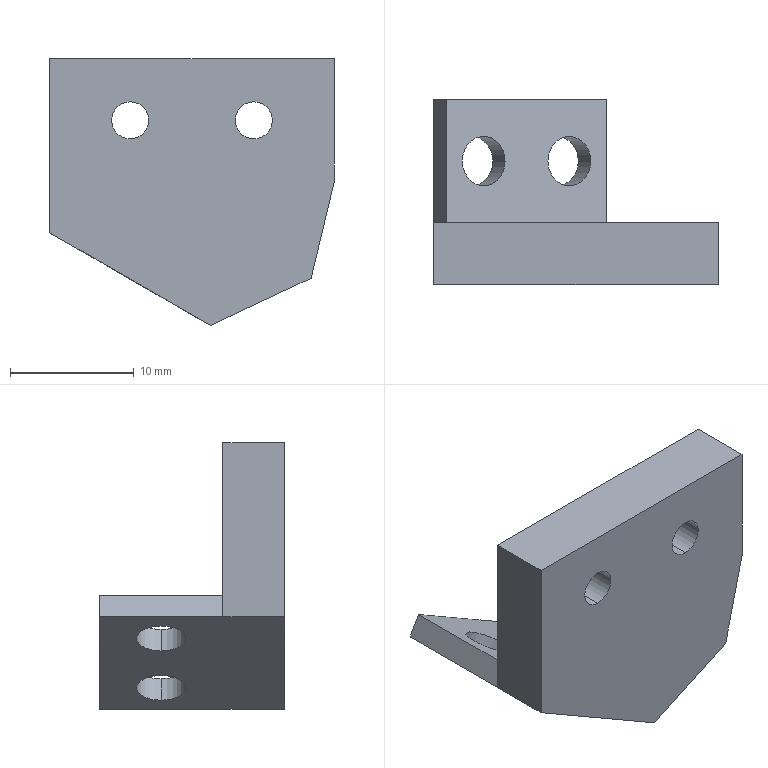Part | SolidWorks | features ICE 3, Extrusion 1 | 1 solid | 20 faces | box 23 x 15 x 21.606 mm | volume 2270 mm3 | plane 12 | cylinder 8 | commonest cylinder face diameters 3 x4 4 x4
STEP:
#1=CARTESIAN_POINT('',(-16.5,0.,-6.5));
#2=VERTEX_POINT('',#1);
#3=CARTESIAN_POINT('',(-16.5,0.,-3.5));
#4=VERTEX_POINT('',#3);
#5=CARTESIAN_POINT('',(-16.5,0.,-5.));
#6=DIRECTION('',(0.,1.,0.));
#7=DIRECTION('',(0.,0.,1.));
#8=AXIS2_PLACEMENT_3D('',#5,#6,#7);
#9=CIRCLE('',#8,1.5);
#10=EDGE_CURVE('',#2,#4,#9,.T.);
#11=ORIENTED_EDGE('',*,*,#10,.F.);
#12=CARTESIAN_POINT('',(-16.5,5.,-6.5));
#13=VERTEX_POINT('',#12);
#14=CARTESIAN_POINT('',(-16.5,0.,-6.5));
#15=DIRECTION('',(0.,1.,0.));
#16=VECTOR('',#15,1000.);
#17=LINE('',#14,#16);
#18=EDGE_CURVE('',#2,#13,#17,.T.);
#19=ORIENTED_EDGE('',*,*,#18,.T.);
#20=CARTESIAN_POINT('',(-16.5,5.,-3.5));
#21=VERTEX_POINT('',#20);
#22=CARTESIAN_POINT('',(-16.5,5.,-5.));
#23=DIRECTION('',(0.,-1.,0.));
#24=DIRECTION('',(0.,0.,-1.));
#25=AXIS2_PLACEMENT_3D('',#22,#23,#24);
#26=CIRCLE('',#25,1.5);
#27=EDGE_CURVE('',#21,#13,#26,.T.);
#28=ORIENTED_EDGE('',*,*,#27,.F.);
#29=CARTESIAN_POINT('',(-16.5,0.,-3.5));
#30=DIRECTION('',(0.,1.,0.));
#31=VECTOR('',#30,1000.);
#32=LINE('',#29,#31);
#33=EDGE_CURVE('',#4,#21,#32,.T.);
#34=ORIENTED_EDGE('',*,*,#33,.F.);
#35=EDGE_LOOP('',(#11,#19,#28,#34));
#36=FACE_OUTER_BOUND('',#35,.T.);
#37=CARTESIAN_POINT('',(-16.5,0.,-5.));
#38=DIRECTION('',(0.,1.,0.));
#39=DIRECTION('',(0.,0.,1.));
#40=AXIS2_PLACEMENT_3D('',#37,#38,#39);
#41=CYLINDRICAL_SURFACE('',#40,1.5);
#42=ADVANCED_FACE('',(#36),#41,.F.);
#43=CARTESIAN_POINT('',(-6.5,0.,-6.5));
#44=VERTEX_POINT('',#43);
#45=CARTESIAN_POINT('',(-6.5,0.,-3.5));
#46=VERTEX_POINT('',#45);
#47=CARTESIAN_POINT('',(-6.5,0.,-5.));
#48=DIRECTION('',(0.,1.,0.));
#49=DIRECTION('',(0.,0.,1.));
#50=AXIS2_PLACEMENT_3D('',#47,#48,#49);
#51=CIRCLE('',#50,1.5);
#52=EDGE_CURVE('',#44,#46,#51,.T.);
#53=ORIENTED_EDGE('',*,*,#52,.F.);
#54=CARTESIAN_POINT('',(-6.5,5.,-6.5));
#55=VERTEX_POINT('',#54);
#56=CARTESIAN_POINT('',(-6.5,0.,-6.5));
#57=DIRECTION('',(0.,1.,0.));
#58=VECTOR('',#57,1000.);
#59=LINE('',#56,#58);
#60=EDGE_CURVE('',#44,#55,#59,.T.);
#61=ORIENTED_EDGE('',*,*,#60,.T.);
#62=CARTESIAN_POINT('',(-6.5,5.,-3.5));
#63=VERTEX_POINT('',#62);
#64=CARTESIAN_POINT('',(-6.5,5.,-5.));
#65=DIRECTION('',(0.,-1.,0.));
#66=DIRECTION('',(0.,0.,-1.));
#67=AXIS2_PLACEMENT_3D('',#64,#65,#66);
#68=CIRCLE('',#67,1.5);
#69=EDGE_CURVE('',#63,#55,#68,.T.);
#70=ORIENTED_EDGE('',*,*,#69,.F.);
#71=CARTESIAN_POINT('',(-6.5,0.,-3.5));
#72=DIRECTION('',(0.,1.,0.));
#73=VECTOR('',#72,1000.);
#74=LINE('',#71,#73);
#75=EDGE_CURVE('',#46,#63,#74,.T.);
#76=ORIENTED_EDGE('',*,*,#75,.F.);
#77=EDGE_LOOP('',(#53,#61,#70,#76));
#78=FACE_OUTER_BOUND('',#77,.T.);
#79=CARTESIAN_POINT('',(-6.5,0.,-5.));
#80=DIRECTION('',(0.,1.,0.));
#81=DIRECTION('',(0.,0.,1.));
#82=AXIS2_PLACEMENT_3D('',#79,#80,#81);
#83=CYLINDRICAL_SURFACE('',#82,1.5);
#84=ADVANCED_FACE('',(#78),#83,.F.);
#85=CARTESIAN_POINT('',(-14.773,10.,-18.856));
#86=VERTEX_POINT('',#85);
#87=CARTESIAN_POINT('',(-11.309,10.,-20.856));
#88=VERTEX_POINT('',#87);
#89=CARTESIAN_POINT('',(-13.041,10.,-19.856));
#90=DIRECTION('',(0.5,0.,0.866));
#91=DIRECTION('',(0.866,0.,-0.5));
#92=AXIS2_PLACEMENT_3D('',#89,#90,#91);
#93=CIRCLE('',#92,2.);
#94=EDGE_CURVE('',#86,#88,#93,.T.);
#95=ORIENTED_EDGE('',*,*,#94,.F.);
#96=CARTESIAN_POINT('',(-13.773,10.,-17.124));
#97=VERTEX_POINT('',#96);
#98=CARTESIAN_POINT('',(-18.02,10.,-24.481));
#99=DIRECTION('',(0.5,0.,0.866));
#100=VECTOR('',#99,1000.);
#101=LINE('',#98,#100);
#102=EDGE_CURVE('',#86,#97,#101,.T.);
#103=ORIENTED_EDGE('',*,*,#102,.T.);
#104=CARTESIAN_POINT('',(-10.309,10.,-19.124));
#105=VERTEX_POINT('',#104);
#106=CARTESIAN_POINT('',(-12.041,10.,-18.124));
#107=DIRECTION('',(-0.5,0.,-0.866));
#108=DIRECTION('',(-0.866,0.,0.5));
#109=AXIS2_PLACEMENT_3D('',#106,#107,#108);
#110=CIRCLE('',#109,2.);
#111=EDGE_CURVE('',#105,#97,#110,.T.);
#112=ORIENTED_EDGE('',*,*,#111,.F.);
#113=CARTESIAN_POINT('',(-14.556,10.,-26.481));
#114=DIRECTION('',(0.5,0.,0.866));
#115=VECTOR('',#114,1000.);
#116=LINE('',#113,#115);
#117=EDGE_CURVE('',#88,#105,#116,.T.);
#118=ORIENTED_EDGE('',*,*,#117,.F.);
#119=EDGE_LOOP('',(#95,#103,#112,#118));
#120=FACE_OUTER_BOUND('',#119,.T.);
#121=CARTESIAN_POINT('',(-16.288,10.,-25.481));
#122=DIRECTION('',(0.5,0.,0.866));
#123=DIRECTION('',(0.866,0.,-0.5));
#124=AXIS2_PLACEMENT_3D('',#121,#122,#123);
#125=CYLINDRICAL_SURFACE('',#124,2.);
#126=ADVANCED_FACE('',(#120),#125,.F.);
#127=CARTESIAN_POINT('',(-21.701,10.,-14.856));
#128=VERTEX_POINT('',#127);
#129=CARTESIAN_POINT('',(-18.237,10.,-16.856));
#130=VERTEX_POINT('',#129);
#131=CARTESIAN_POINT('',(-19.969,10.,-15.856));
#132=DIRECTION('',(0.5,0.,0.866));
#133=DIRECTION('',(0.866,0.,-0.5));
#134=AXIS2_PLACEMENT_3D('',#131,#132,#133);
#135=CIRCLE('',#134,2.);
#136=EDGE_CURVE('',#128,#130,#135,.T.);
#137=ORIENTED_EDGE('',*,*,#136,.F.);
#138=CARTESIAN_POINT('',(-20.701,10.,-13.124));
#139=VERTEX_POINT('',#138);
#140=CARTESIAN_POINT('',(-24.949,10.,-20.481));
#141=DIRECTION('',(0.5,0.,0.866));
#142=VECTOR('',#141,1000.);
#143=LINE('',#140,#142);
#144=EDGE_CURVE('',#128,#139,#143,.T.);
#145=ORIENTED_EDGE('',*,*,#144,.T.);
#146=CARTESIAN_POINT('',(-17.237,10.,-15.124));
#147=VERTEX_POINT('',#146);
#148=CARTESIAN_POINT('',(-18.969,10.,-14.124));
#149=DIRECTION('',(-0.5,0.,-0.866));
#150=DIRECTION('',(-0.866,0.,0.5));
#151=AXIS2_PLACEMENT_3D('',#148,#149,#150);
#152=CIRCLE('',#151,2.);
#153=EDGE_CURVE('',#147,#139,#152,.T.);
#154=ORIENTED_EDGE('',*,*,#153,.F.);
#155=CARTESIAN_POINT('',(-21.484,10.,-22.481));
#156=DIRECTION('',(0.5,0.,0.866));
#157=VECTOR('',#156,1000.);
#158=LINE('',#155,#157);
#159=EDGE_CURVE('',#130,#147,#158,.T.);
#160=ORIENTED_EDGE('',*,*,#159,.F.);
#161=EDGE_LOOP('',(#137,#145,#154,#160));
#162=FACE_OUTER_BOUND('',#161,.T.);
#163=CARTESIAN_POINT('',(-23.217,10.,-21.481));
#164=DIRECTION('',(0.5,0.,0.866));
#165=DIRECTION('',(0.866,0.,-0.5));
#166=AXIS2_PLACEMENT_3D('',#163,#164,#165);
#167=CYLINDRICAL_SURFACE('',#166,2.);
#168=ADVANCED_FACE('',(#162),#167,.F.);
#169=ORIENTED_EDGE('',*,*,#27,.T.);
#170=CARTESIAN_POINT('',(-16.5,5.,-5.));
#171=DIRECTION('',(0.,-1.,0.));
#172=DIRECTION('',(0.,0.,-1.));
#173=AXIS2_PLACEMENT_3D('',#170,#171,#172);
#174=CIRCLE('',#173,1.5);
#175=EDGE_CURVE('',#13,#21,#174,.T.);
#176=ORIENTED_EDGE('',*,*,#175,.T.);
#177=EDGE_LOOP('',(#169,#176));
#178=FACE_BOUND('',#177,.T.);
#179=ORIENTED_EDGE('',*,*,#69,.T.);
#180=CARTESIAN_POINT('',(-6.5,5.,-5.));
#181=DIRECTION('',(0.,-1.,0.));
#182=DIRECTION('',(0.,0.,-1.));
#183=AXIS2_PLACEMENT_3D('',#180,#181,#182);
#184=CIRCLE('',#183,1.5);
#185=EDGE_CURVE('',#55,#63,#184,.T.);
#186=ORIENTED_EDGE('',*,*,#185,.T.);
#187=EDGE_LOOP('',(#179,#186));
#188=FACE_BOUND('',#187,.T.);
#189=CARTESIAN_POINT('',(-9.01,5.,-19.874));
#190=VERTEX_POINT('',#189);
#191=CARTESIAN_POINT('',(-10.01,5.,-21.606));
#192=VERTEX_POINT('',#191);
#193=CARTESIAN_POINT('',(-10.01,5.,-21.606));
#194=DIRECTION('',(-0.5,0.,-0.866));
#195=VECTOR('',#194,1000.);
#196=LINE('',#193,#195);
#197=EDGE_CURVE('',#190,#192,#196,.T.);
#198=ORIENTED_EDGE('',*,*,#197,.F.);
#199=CARTESIAN_POINT('',(-22.,5.,-12.374));
#200=VERTEX_POINT('',#199);
#201=CARTESIAN_POINT('',(-22.,5.,-12.374));
#202=DIRECTION('',(0.866,0.,-0.5));
#203=VECTOR('',#202,1000.);
#204=LINE('',#201,#203);
#205=EDGE_CURVE('',#200,#190,#204,.T.);
#206=ORIENTED_EDGE('',*,*,#205,.F.);
#207=CARTESIAN_POINT('',(-23.,5.,-14.106));
#208=VERTEX_POINT('',#207);
#209=CARTESIAN_POINT('',(-23.,5.,-14.106));
#210=DIRECTION('',(0.5,0.,0.866));
#211=VECTOR('',#210,1000.);
#212=LINE('',#209,#211);
#213=EDGE_CURVE('',#208,#200,#212,.T.);
#214=ORIENTED_EDGE('',*,*,#213,.F.);
#215=CARTESIAN_POINT('',(-23.,5.,0.));
#216=VERTEX_POINT('',#215);
#217=CARTESIAN_POINT('',(-23.,5.,0.));
#218=DIRECTION('',(0.,0.,1.));
#219=VECTOR('',#218,1000.);
#220=LINE('',#217,#219);
#221=EDGE_CURVE('',#208,#216,#220,.T.);
#222=ORIENTED_EDGE('',*,*,#221,.T.);
#223=CARTESIAN_POINT('',(0.,5.,0.));
#224=VERTEX_POINT('',#223);
#225=CARTESIAN_POINT('',(0.,5.,0.));
#226=DIRECTION('',(1.,0.,0.));
#227=VECTOR('',#226,1000.);
#228=LINE('',#225,#227);
#229=EDGE_CURVE('',#216,#224,#228,.T.);
#230=ORIENTED_EDGE('',*,*,#229,.T.);
#231=CARTESIAN_POINT('',(0.,5.,-10.));
#232=VERTEX_POINT('',#231);
#233=CARTESIAN_POINT('',(0.,5.,-10.));
#234=DIRECTION('',(0.,0.,-1.));
#235=VECTOR('',#234,1000.);
#236=LINE('',#233,#235);
#237=EDGE_CURVE('',#224,#232,#236,.T.);
#238=ORIENTED_EDGE('',*,*,#237,.T.);
#239=CARTESIAN_POINT('',(-1.863,5.,-17.78));
#240=VERTEX_POINT('',#239);
#241=CARTESIAN_POINT('',(-1.863,5.,-17.78));
#242=DIRECTION('',(-0.2329,0.,-0.9725));
#243=VECTOR('',#242,1000.);
#244=LINE('',#241,#243);
#245=EDGE_CURVE('',#232,#240,#244,.T.);
#246=ORIENTED_EDGE('',*,*,#245,.T.);
#247=CARTESIAN_POINT('',(-10.01,5.,-21.606));
#248=DIRECTION('',(-0.9052,0.,-0.4251));
#249=VECTOR('',#248,1000.);
#250=LINE('',#247,#249);
#251=EDGE_CURVE('',#240,#192,#250,.T.);
#252=ORIENTED_EDGE('',*,*,#251,.T.);
#253=EDGE_LOOP('',(#198,#206,#214,#222,#230,#238,#246,#252));
#254=FACE_OUTER_BOUND('',#253,.T.);
#255=CARTESIAN_POINT('',(0.,5.,0.));
#256=DIRECTION('',(0.,-1.,0.));
#257=DIRECTION('',(0.,0.,-1.));
#258=AXIS2_PLACEMENT_3D('',#255,#256,#257);
#259=PLANE('',#258);
#260=ADVANCED_FACE('',(#178,#188,#254),#259,.F.);
#261=CARTESIAN_POINT('',(0.,0.,0.));
#262=VERTEX_POINT('',#261);
#263=CARTESIAN_POINT('',(0.,0.,-10.));
#264=VERTEX_POINT('',#263);
#265=CARTESIAN_POINT('',(0.,0.,-10.));
#266=DIRECTION('',(0.,0.,-1.));
#267=VECTOR('',#266,1000.);
#268=LINE('',#265,#267);
#269=EDGE_CURVE('',#262,#264,#268,.T.);
#270=ORIENTED_EDGE('',*,*,#269,.T.);
#271=CARTESIAN_POINT('',(0.,5.,-10.));
#272=DIRECTION('',(0.,-1.,0.));
#273=VECTOR('',#272,1000.);
#274=LINE('',#271,#273);
#275=EDGE_CURVE('',#232,#264,#274,.T.);
#276=ORIENTED_EDGE('',*,*,#275,.F.);
#277=ORIENTED_EDGE('',*,*,#237,.F.);
#278=CARTESIAN_POINT('',(0.,5.,0.));
#279=DIRECTION('',(0.,-1.,0.));
#280=VECTOR('',#279,1000.);
#281=LINE('',#278,#280);
#282=EDGE_CURVE('',#224,#262,#281,.T.);
#283=ORIENTED_EDGE('',*,*,#282,.T.);
#284=EDGE_LOOP('',(#270,#276,#277,#283));
#285=FACE_OUTER_BOUND('',#284,.T.);
#286=CARTESIAN_POINT('',(0.,5.,-10.));
#287=DIRECTION('',(-1.,0.,0.));
#288=DIRECTION('',(0.,0.,1.));
#289=AXIS2_PLACEMENT_3D('',#286,#287,#288);
#290=PLANE('',#289);
#291=ADVANCED_FACE('',(#285),#290,.F.);
#292=CARTESIAN_POINT('',(-1.863,0.,-17.78));
#293=VERTEX_POINT('',#292);
#294=CARTESIAN_POINT('',(-1.863,0.,-17.78));
#295=DIRECTION('',(-0.2329,0.,-0.9725));
#296=VECTOR('',#295,1000.);
#297=LINE('',#294,#296);
#298=EDGE_CURVE('',#264,#293,#297,.T.);
#299=ORIENTED_EDGE('',*,*,#298,.T.);
#300=CARTESIAN_POINT('',(-1.863,5.,-17.78));
#301=DIRECTION('',(0.,-1.,0.));
#302=VECTOR('',#301,1000.);
#303=LINE('',#300,#302);
#304=EDGE_CURVE('',#240,#293,#303,.T.);
#305=ORIENTED_EDGE('',*,*,#304,.F.);
#306=ORIENTED_EDGE('',*,*,#245,.F.);
#307=ORIENTED_EDGE('',*,*,#275,.T.);
#308=EDGE_LOOP('',(#299,#305,#306,#307));
#309=FACE_OUTER_BOUND('',#308,.T.);
#310=CARTESIAN_POINT('',(-1.863,5.,-17.78));
#311=DIRECTION('',(-0.9725,0.,0.2329));
#312=DIRECTION('',(0.2329,0.,0.9725));
#313=AXIS2_PLACEMENT_3D('',#310,#311,#312);
#314=PLANE('',#313);
#315=ADVANCED_FACE('',(#309),#314,.F.);
#316=CARTESIAN_POINT('',(-10.01,0.,-21.606));
#317=VERTEX_POINT('',#316);
#318=CARTESIAN_POINT('',(-10.01,0.,-21.606));
#319=DIRECTION('',(-0.9052,0.,-0.4251));
#320=VECTOR('',#319,1000.);
#321=LINE('',#318,#320);
#322=EDGE_CURVE('',#293,#317,#321,.T.);
#323=ORIENTED_EDGE('',*,*,#322,.T.);
#324=CARTESIAN_POINT('',(-10.01,5.,-21.606));
#325=DIRECTION('',(0.,-1.,0.));
#326=VECTOR('',#325,1000.);
#327=LINE('',#324,#326);
#328=EDGE_CURVE('',#192,#317,#327,.T.);
#329=ORIENTED_EDGE('',*,*,#328,.F.);
#330=ORIENTED_EDGE('',*,*,#251,.F.);
#331=ORIENTED_EDGE('',*,*,#304,.T.);
#332=EDGE_LOOP('',(#323,#329,#330,#331));
#333=FACE_OUTER_BOUND('',#332,.T.);
#334=CARTESIAN_POINT('',(-10.01,5.,-21.606));
#335=DIRECTION('',(-0.4251,0.,0.9052));
#336=DIRECTION('',(0.9052,0.,0.4251));
#337=AXIS2_PLACEMENT_3D('',#334,#335,#336);
#338=PLANE('',#337);
#339=ADVANCED_FACE('',(#333),#338,.F.);
#340=CARTESIAN_POINT('',(-13.041,10.,-19.856));
#341=DIRECTION('',(0.5,0.,0.866));
#342=DIRECTION('',(0.866,0.,-0.5));
#343=AXIS2_PLACEMENT_3D('',#340,#341,#342);
#344=CIRCLE('',#343,2.);
#345=EDGE_CURVE('',#88,#86,#344,.T.);
#346=ORIENTED_EDGE('',*,*,#345,.T.);
#347=ORIENTED_EDGE('',*,*,#94,.T.);
#348=EDGE_LOOP('',(#346,#347));
#349=FACE_BOUND('',#348,.T.);
#350=CARTESIAN_POINT('',(-19.969,10.,-15.856));
#351=DIRECTION('',(0.5,0.,0.866));
#352=DIRECTION('',(0.866,0.,-0.5));
#353=AXIS2_PLACEMENT_3D('',#350,#351,#352);
#354=CIRCLE('',#353,2.);
#355=EDGE_CURVE('',#130,#128,#354,.T.);
#356=ORIENTED_EDGE('',*,*,#355,.T.);
#357=ORIENTED_EDGE('',*,*,#136,.T.);
#358=EDGE_LOOP('',(#356,#357));
#359=FACE_BOUND('',#358,.T.);
#360=CARTESIAN_POINT('',(-23.,0.,-14.106));
#361=VERTEX_POINT('',#360);
#362=CARTESIAN_POINT('',(-23.,0.,-14.106));
#363=DIRECTION('',(-0.866,0.,0.5));
#364=VECTOR('',#363,1000.);
#365=LINE('',#362,#364);
#366=EDGE_CURVE('',#317,#361,#365,.T.);
#367=ORIENTED_EDGE('',*,*,#366,.T.);
#368=CARTESIAN_POINT('',(-23.,5.,-14.106));
#369=DIRECTION('',(0.,-1.,0.));
#370=VECTOR('',#369,1000.);
#371=LINE('',#368,#370);
#372=EDGE_CURVE('',#208,#361,#371,.T.);
#373=ORIENTED_EDGE('',*,*,#372,.F.);
#374=CARTESIAN_POINT('',(-23.,15.,-14.106));
#375=VERTEX_POINT('',#374);
#376=CARTESIAN_POINT('',(-23.,15.,-14.106));
#377=DIRECTION('',(0.,-1.,0.));
#378=VECTOR('',#377,1000.);
#379=LINE('',#376,#378);
#380=EDGE_CURVE('',#375,#208,#379,.T.);
#381=ORIENTED_EDGE('',*,*,#380,.F.);
#382=CARTESIAN_POINT('',(-10.01,15.,-21.606));
#383=VERTEX_POINT('',#382);
#384=CARTESIAN_POINT('',(-10.01,15.,-21.606));
#385=DIRECTION('',(-0.866,0.,0.5));
#386=VECTOR('',#385,1000.);
#387=LINE('',#384,#386);
#388=EDGE_CURVE('',#383,#375,#387,.T.);
#389=ORIENTED_EDGE('',*,*,#388,.F.);
#390=CARTESIAN_POINT('',(-10.01,15.,-21.606));
#391=DIRECTION('',(0.,-1.,0.));
#392=VECTOR('',#391,1000.);
#393=LINE('',#390,#392);
#394=EDGE_CURVE('',#383,#192,#393,.T.);
#395=ORIENTED_EDGE('',*,*,#394,.T.);
#396=ORIENTED_EDGE('',*,*,#328,.T.);
#397=EDGE_LOOP('',(#367,#373,#381,#389,#395,#396));
#398=FACE_OUTER_BOUND('',#397,.T.);
#399=CARTESIAN_POINT('',(-23.,5.,-14.106));
#400=DIRECTION('',(0.5,0.,0.866));
#401=DIRECTION('',(0.866,0.,-0.5));
#402=AXIS2_PLACEMENT_3D('',#399,#400,#401);
#403=PLANE('',#402);
#404=ADVANCED_FACE('',(#349,#359,#398),#403,.F.);
#405=CARTESIAN_POINT('',(-23.,0.,0.));
#406=VERTEX_POINT('',#405);
#407=CARTESIAN_POINT('',(-23.,0.,0.));
#408=DIRECTION('',(0.,0.,1.));
#409=VECTOR('',#408,1000.);
#410=LINE('',#407,#409);
#411=EDGE_CURVE('',#361,#406,#410,.T.);
#412=ORIENTED_EDGE('',*,*,#411,.T.);
#413=CARTESIAN_POINT('',(-23.,5.,0.));
#414=DIRECTION('',(0.,-1.,0.));
#415=VECTOR('',#414,1000.);
#416=LINE('',#413,#415);
#417=EDGE_CURVE('',#216,#406,#416,.T.);
#418=ORIENTED_EDGE('',*,*,#417,.F.);
#419=ORIENTED_EDGE('',*,*,#221,.F.);
#420=ORIENTED_EDGE('',*,*,#372,.T.);
#421=EDGE_LOOP('',(#412,#418,#419,#420));
#422=FACE_OUTER_BOUND('',#421,.T.);
#423=CARTESIAN_POINT('',(-23.,5.,0.));
#424=DIRECTION('',(1.,0.,0.));
#425=DIRECTION('',(0.,0.,-1.));
#426=AXIS2_PLACEMENT_3D('',#423,#424,#425);
#427=PLANE('',#426);
#428=ADVANCED_FACE('',(#422),#427,.F.);
#429=CARTESIAN_POINT('',(0.,0.,0.));
#430=DIRECTION('',(1.,0.,0.));
#431=VECTOR('',#430,1000.);
#432=LINE('',#429,#431);
#433=EDGE_CURVE('',#406,#262,#432,.T.);
#434=ORIENTED_EDGE('',*,*,#433,.T.);
#435=ORIENTED_EDGE('',*,*,#282,.F.);
#436=ORIENTED_EDGE('',*,*,#229,.F.);
#437=ORIENTED_EDGE('',*,*,#417,.T.);
#438=EDGE_LOOP('',(#434,#435,#436,#437));
#439=FACE_OUTER_BOUND('',#438,.T.);
#440=CARTESIAN_POINT('',(0.,5.,0.));
#441=DIRECTION('',(0.,0.,-1.));
#442=DIRECTION('',(-1.,0.,0.));
#443=AXIS2_PLACEMENT_3D('',#440,#441,#442);
#444=PLANE('',#443);
#445=ADVANCED_FACE('',(#439),#444,.F.);
#446=CARTESIAN_POINT('',(-16.5,0.,-5.));
#447=DIRECTION('',(0.,1.,0.));
#448=DIRECTION('',(0.,0.,1.));
#449=AXIS2_PLACEMENT_3D('',#446,#447,#448);
#450=CIRCLE('',#449,1.5);
#451=EDGE_CURVE('',#4,#2,#450,.T.);
#452=ORIENTED_EDGE('',*,*,#451,.T.);
#453=ORIENTED_EDGE('',*,*,#10,.T.);
#454=EDGE_LOOP('',(#452,#453));
#455=FACE_BOUND('',#454,.T.);
#456=CARTESIAN_POINT('',(-6.5,0.,-5.));
#457=DIRECTION('',(0.,1.,0.));
#458=DIRECTION('',(0.,0.,1.));
#459=AXIS2_PLACEMENT_3D('',#456,#457,#458);
#460=CIRCLE('',#459,1.5);
#461=EDGE_CURVE('',#46,#44,#460,.T.);
#462=ORIENTED_EDGE('',*,*,#461,.T.);
#463=ORIENTED_EDGE('',*,*,#52,.T.);
#464=EDGE_LOOP('',(#462,#463));
#465=FACE_BOUND('',#464,.T.);
#466=ORIENTED_EDGE('',*,*,#269,.F.);
#467=ORIENTED_EDGE('',*,*,#433,.F.);
#468=ORIENTED_EDGE('',*,*,#411,.F.);
#469=ORIENTED_EDGE('',*,*,#366,.F.);
#470=ORIENTED_EDGE('',*,*,#322,.F.);
#471=ORIENTED_EDGE('',*,*,#298,.F.);
#472=EDGE_LOOP('',(#466,#467,#468,#469,#470,#471));
#473=FACE_OUTER_BOUND('',#472,.T.);
#474=CARTESIAN_POINT('',(0.,0.,0.));
#475=DIRECTION('',(0.,-1.,0.));
#476=DIRECTION('',(0.,0.,-1.));
#477=AXIS2_PLACEMENT_3D('',#474,#475,#476);
#478=PLANE('',#477);
#479=ADVANCED_FACE('',(#455,#465,#473),#478,.T.);
#480=ORIENTED_EDGE('',*,*,#197,.T.);
#481=ORIENTED_EDGE('',*,*,#394,.F.);
#482=CARTESIAN_POINT('',(-9.01,15.,-19.874));
#483=VERTEX_POINT('',#482);
#484=CARTESIAN_POINT('',(-10.01,15.,-21.606));
#485=DIRECTION('',(-0.5,0.,-0.866));
#486=VECTOR('',#485,1000.);
#487=LINE('',#484,#486);
#488=EDGE_CURVE('',#483,#383,#487,.T.);
#489=ORIENTED_EDGE('',*,*,#488,.F.);
#490=CARTESIAN_POINT('',(-9.01,15.,-19.874));
#491=DIRECTION('',(0.,-1.,0.));
#492=VECTOR('',#491,1000.);
#493=LINE('',#490,#492);
#494=EDGE_CURVE('',#483,#190,#493,.T.);
#495=ORIENTED_EDGE('',*,*,#494,.T.);
#496=EDGE_LOOP('',(#480,#481,#489,#495));
#497=FACE_OUTER_BOUND('',#496,.T.);
#498=CARTESIAN_POINT('',(-10.01,15.,-21.606));
#499=DIRECTION('',(-0.866,0.,0.5));
#500=DIRECTION('',(0.5,0.,0.866));
#501=AXIS2_PLACEMENT_3D('',#498,#499,#500);
#502=PLANE('',#501);
#503=ADVANCED_FACE('',(#497),#502,.F.);
#504=ORIENTED_EDGE('',*,*,#213,.T.);
#505=CARTESIAN_POINT('',(-22.,15.,-12.374));
#506=VERTEX_POINT('',#505);
#507=CARTESIAN_POINT('',(-22.,15.,-12.374));
#508=DIRECTION('',(0.,-1.,0.));
#509=VECTOR('',#508,1000.);
#510=LINE('',#507,#509);
#511=EDGE_CURVE('',#506,#200,#510,.T.);
#512=ORIENTED_EDGE('',*,*,#511,.F.);
#513=CARTESIAN_POINT('',(-23.,15.,-14.106));
#514=DIRECTION('',(0.5,0.,0.866));
#515=VECTOR('',#514,1000.);
#516=LINE('',#513,#515);
#517=EDGE_CURVE('',#375,#506,#516,.T.);
#518=ORIENTED_EDGE('',*,*,#517,.F.);
#519=ORIENTED_EDGE('',*,*,#380,.T.);
#520=EDGE_LOOP('',(#504,#512,#518,#519));
#521=FACE_OUTER_BOUND('',#520,.T.);
#522=CARTESIAN_POINT('',(-23.,15.,-14.106));
#523=DIRECTION('',(0.866,0.,-0.5));
#524=DIRECTION('',(-0.5,0.,-0.866));
#525=AXIS2_PLACEMENT_3D('',#522,#523,#524);
#526=PLANE('',#525);
#527=ADVANCED_FACE('',(#521),#526,.F.);
#528=ORIENTED_EDGE('',*,*,#111,.T.);
#529=CARTESIAN_POINT('',(-12.041,10.,-18.124));
#530=DIRECTION('',(-0.5,0.,-0.866));
#531=DIRECTION('',(-0.866,0.,0.5));
#532=AXIS2_PLACEMENT_3D('',#529,#530,#531);
#533=CIRCLE('',#532,2.);
#534=EDGE_CURVE('',#97,#105,#533,.T.);
#535=ORIENTED_EDGE('',*,*,#534,.T.);
#536=EDGE_LOOP('',(#528,#535));
#537=FACE_BOUND('',#536,.T.);
#538=ORIENTED_EDGE('',*,*,#153,.T.);
#539=CARTESIAN_POINT('',(-18.969,10.,-14.124));
#540=DIRECTION('',(-0.5,0.,-0.866));
#541=DIRECTION('',(-0.866,0.,0.5));
#542=AXIS2_PLACEMENT_3D('',#539,#540,#541);
#543=CIRCLE('',#542,2.);
#544=EDGE_CURVE('',#139,#147,#543,.T.);
#545=ORIENTED_EDGE('',*,*,#544,.T.);
#546=EDGE_LOOP('',(#538,#545));
#547=FACE_BOUND('',#546,.T.);
#548=ORIENTED_EDGE('',*,*,#205,.T.);
#549=ORIENTED_EDGE('',*,*,#494,.F.);
#550=CARTESIAN_POINT('',(-22.,15.,-12.374));
#551=DIRECTION('',(0.866,0.,-0.5));
#552=VECTOR('',#551,1000.);
#553=LINE('',#550,#552);
#554=EDGE_CURVE('',#506,#483,#553,.T.);
#555=ORIENTED_EDGE('',*,*,#554,.F.);
#556=ORIENTED_EDGE('',*,*,#511,.T.);
#557=EDGE_LOOP('',(#548,#549,#555,#556));
#558=FACE_OUTER_BOUND('',#557,.T.);
#559=CARTESIAN_POINT('',(-22.,15.,-12.374));
#560=DIRECTION('',(-0.5,0.,-0.866));
#561=DIRECTION('',(-0.866,0.,0.5));
#562=AXIS2_PLACEMENT_3D('',#559,#560,#561);
#563=PLANE('',#562);
#564=ADVANCED_FACE('',(#537,#547,#558),#563,.F.);
#565=ORIENTED_EDGE('',*,*,#488,.T.);
#566=ORIENTED_EDGE('',*,*,#388,.T.);
#567=ORIENTED_EDGE('',*,*,#517,.T.);
#568=ORIENTED_EDGE('',*,*,#554,.T.);
#569=EDGE_LOOP('',(#565,#566,#567,#568));
#570=FACE_OUTER_BOUND('',#569,.T.);
#571=CARTESIAN_POINT('',(0.,15.,0.));
#572=DIRECTION('',(0.,1.,0.));
#573=DIRECTION('',(0.,0.,1.));
#574=AXIS2_PLACEMENT_3D('',#571,#572,#573);
#575=PLANE('',#574);
#576=ADVANCED_FACE('',(#570),#575,.T.);
#577=ORIENTED_EDGE('',*,*,#144,.F.);
#578=ORIENTED_EDGE('',*,*,#355,.F.);
#579=ORIENTED_EDGE('',*,*,#159,.T.);
#580=ORIENTED_EDGE('',*,*,#544,.F.);
#581=EDGE_LOOP('',(#577,#578,#579,#580));
#582=FACE_OUTER_BOUND('',#581,.T.);
#583=CARTESIAN_POINT('',(-23.217,10.,-21.481));
#584=DIRECTION('',(0.5,0.,0.866));
#585=DIRECTION('',(0.866,0.,-0.5));
#586=AXIS2_PLACEMENT_3D('',#583,#584,#585);
#587=CYLINDRICAL_SURFACE('',#586,2.);
#588=ADVANCED_FACE('',(#582),#587,.F.);
#589=ORIENTED_EDGE('',*,*,#102,.F.);
#590=ORIENTED_EDGE('',*,*,#345,.F.);
#591=ORIENTED_EDGE('',*,*,#117,.T.);
#592=ORIENTED_EDGE('',*,*,#534,.F.);
#593=EDGE_LOOP('',(#589,#590,#591,#592));
#594=FACE_OUTER_BOUND('',#593,.T.);
#595=CARTESIAN_POINT('',(-16.288,10.,-25.481));
#596=DIRECTION('',(0.5,0.,0.866));
#597=DIRECTION('',(0.866,0.,-0.5));
#598=AXIS2_PLACEMENT_3D('',#595,#596,#597);
#599=CYLINDRICAL_SURFACE('',#598,2.);
#600=ADVANCED_FACE('',(#594),#599,.F.);
#601=ORIENTED_EDGE('',*,*,#60,.F.);
#602=ORIENTED_EDGE('',*,*,#461,.F.);
#603=ORIENTED_EDGE('',*,*,#75,.T.);
#604=ORIENTED_EDGE('',*,*,#185,.F.);
#605=EDGE_LOOP('',(#601,#602,#603,#604));
#606=FACE_OUTER_BOUND('',#605,.T.);
#607=CARTESIAN_POINT('',(-6.5,0.,-5.));
#608=DIRECTION('',(0.,1.,0.));
#609=DIRECTION('',(0.,0.,1.));
#610=AXIS2_PLACEMENT_3D('',#607,#608,#609);
#611=CYLINDRICAL_SURFACE('',#610,1.5);
#612=ADVANCED_FACE('',(#606),#611,.F.);
#613=ORIENTED_EDGE('',*,*,#18,.F.);
#614=ORIENTED_EDGE('',*,*,#451,.F.);
#615=ORIENTED_EDGE('',*,*,#33,.T.);
#616=ORIENTED_EDGE('',*,*,#175,.F.);
#617=EDGE_LOOP('',(#613,#614,#615,#616));
#618=FACE_OUTER_BOUND('',#617,.T.);
#619=CARTESIAN_POINT('',(-16.5,0.,-5.));
#620=DIRECTION('',(0.,1.,0.));
#621=DIRECTION('',(0.,0.,1.));
#622=AXIS2_PLACEMENT_3D('',#619,#620,#621);
#623=CYLINDRICAL_SURFACE('',#622,1.5);
#624=ADVANCED_FACE('',(#618),#623,.F.);
#625=CLOSED_SHELL('',(#42,#84,#126,#168,#260,#291,#315,#339,#404,#428,#445,#479,#503,#527,#564,#576,#588,#600,#612,#624));
#626=MANIFOLD_SOLID_BREP('',#625);
#627=CARTESIAN_POINT('',(0.,0.,0.));
#628=DIRECTION('',(0.,0.,1.));
#629=DIRECTION('',(1.,0.,0.));
#630=AXIS2_PLACEMENT_3D('',#627,#628,#629);
#631=(LENGTH_UNIT()NAMED_UNIT(*)SI_UNIT(.MILLI.,.METRE.));
#632=UNCERTAINTY_MEASURE_WITH_UNIT(LENGTH_MEASURE(0.00001),#631,'','');
#633=(NAMED_UNIT(*)PLANE_ANGLE_UNIT()SI_UNIT($,.RADIAN.));
#634=(NAMED_UNIT(*)SI_UNIT($,.STERADIAN.)SOLID_ANGLE_UNIT());
#635=(GEOMETRIC_REPRESENTATION_CONTEXT(3)GLOBAL_UNCERTAINTY_ASSIGNED_CONTEXT((#632))GLOBAL_UNIT_ASSIGNED_CONTEXT((#631,#633,#634))REPRESENTATION_CONTEXT('',''));
#636=ADVANCED_BREP_SHAPE_REPRESENTATION('',(#626,#630),#635);